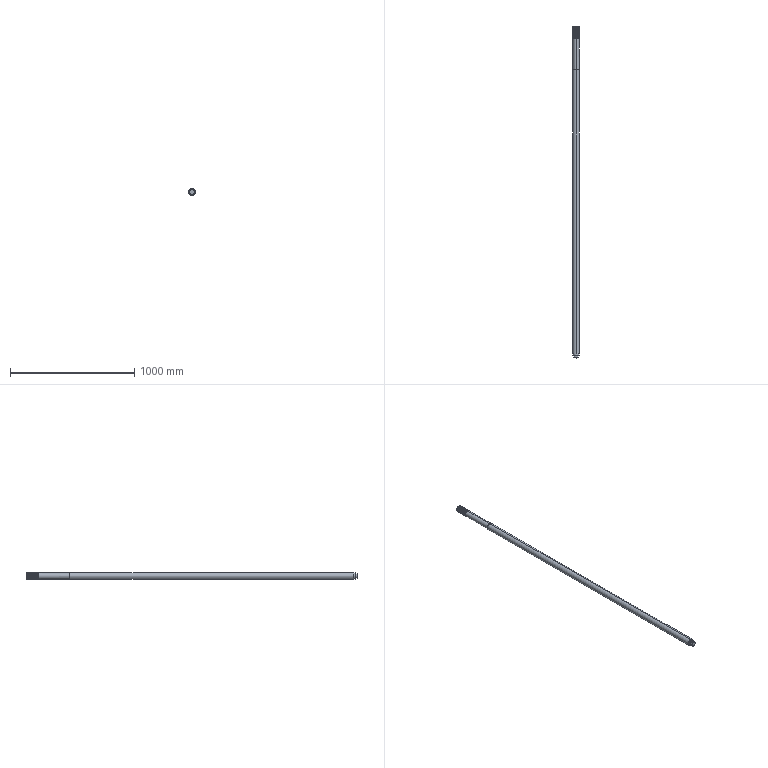Part | SolidWorks | features BaseBody 1 | 1 solid | 166 faces | box 55 x 2670 x 55 mm | volume 6167636 mm3 | cylinder 143 | cone 12 | plane 8 | spline 3 | commonest cylinder face diameters 50 x137 34 x2 40 x2 55 x2